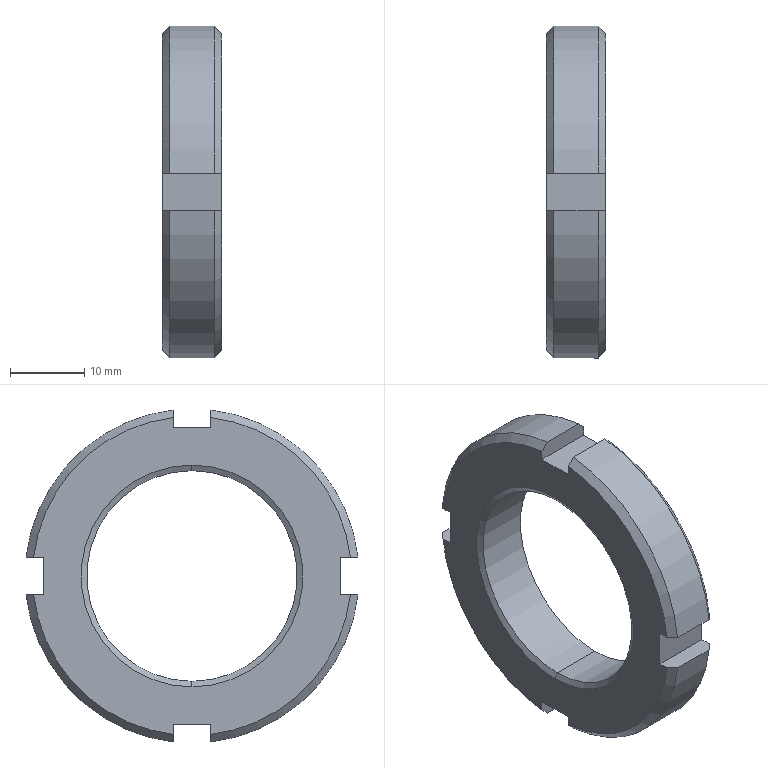Part | SolidWorks | features BaseBody 1 | 1 solid | 32 faces | box 8 x 44.721 x 44.721 mm | volume 7123 mm3 | plane 14 | cone 12 | cylinder 6 | commonest cylinder face diameters 45 x4 28.376 x2
STEP:
#1=CARTESIAN_POINT('',(0.433,0.,-14.188));
#2=VERTEX_POINT('',#1);
#3=CARTESIAN_POINT('',(0.433,0.,14.188));
#4=VERTEX_POINT('',#3);
#5=CARTESIAN_POINT('',(0.433,0.,0.));
#6=DIRECTION('',(-1.,0.,0.));
#7=DIRECTION('',(0.,0.,-1.));
#8=AXIS2_PLACEMENT_3D('',#5,#6,#7);
#9=CIRCLE('',#8,14.188);
#10=EDGE_CURVE('',#2,#4,#9,.T.);
#11=ORIENTED_EDGE('',*,*,#10,.F.);
#12=CARTESIAN_POINT('',(0.,0.,-14.938));
#13=VERTEX_POINT('',#12);
#14=CARTESIAN_POINT('',(0.,0.,-14.938));
#15=DIRECTION('',(-0.5,0.,-0.866));
#16=VECTOR('',#15,1000.);
#17=LINE('',#14,#16);
#18=EDGE_CURVE('',#2,#13,#17,.T.);
#19=ORIENTED_EDGE('',*,*,#18,.T.);
#20=CARTESIAN_POINT('',(0.,0.,14.938));
#21=VERTEX_POINT('',#20);
#22=CARTESIAN_POINT('',(0.,0.,0.));
#23=DIRECTION('',(1.,0.,0.));
#24=DIRECTION('',(0.,0.,1.));
#25=AXIS2_PLACEMENT_3D('',#22,#23,#24);
#26=CIRCLE('',#25,14.938);
#27=EDGE_CURVE('',#21,#13,#26,.T.);
#28=ORIENTED_EDGE('',*,*,#27,.F.);
#29=CARTESIAN_POINT('',(0.,0.,14.938));
#30=DIRECTION('',(-0.5,0.,0.866));
#31=VECTOR('',#30,1000.);
#32=LINE('',#29,#31);
#33=EDGE_CURVE('',#4,#21,#32,.T.);
#34=ORIENTED_EDGE('',*,*,#33,.F.);
#35=EDGE_LOOP('',(#11,#19,#28,#34));
#36=FACE_OUTER_BOUND('',#35,.T.);
#37=CARTESIAN_POINT('',(0.,0.,0.));
#38=DIRECTION('',(-1.,0.,0.));
#39=DIRECTION('',(0.,0.,1.));
#40=AXIS2_PLACEMENT_3D('',#37,#38,#39);
#41=CONICAL_SURFACE('',#40,14.938,1.047);
#42=ADVANCED_FACE('',(#36),#41,.F.);
#43=CARTESIAN_POINT('',(7.567,0.,-14.188));
#44=VERTEX_POINT('',#43);
#45=CARTESIAN_POINT('',(7.567,0.,14.188));
#46=VERTEX_POINT('',#45);
#47=CARTESIAN_POINT('',(7.567,0.,0.));
#48=DIRECTION('',(-1.,0.,0.));
#49=DIRECTION('',(0.,0.,1.));
#50=AXIS2_PLACEMENT_3D('',#47,#48,#49);
#51=CIRCLE('',#50,14.188);
#52=EDGE_CURVE('',#44,#46,#51,.T.);
#53=ORIENTED_EDGE('',*,*,#52,.F.);
#54=CARTESIAN_POINT('',(64.14,0.,-14.188));
#55=DIRECTION('',(-1.,0.,0.));
#56=VECTOR('',#55,1000.);
#57=LINE('',#54,#56);
#58=EDGE_CURVE('',#44,#2,#57,.T.);
#59=ORIENTED_EDGE('',*,*,#58,.T.);
#60=ORIENTED_EDGE('',*,*,#10,.T.);
#61=CARTESIAN_POINT('',(64.14,0.,14.188));
#62=DIRECTION('',(-1.,0.,0.));
#63=VECTOR('',#62,1000.);
#64=LINE('',#61,#63);
#65=EDGE_CURVE('',#46,#4,#64,.T.);
#66=ORIENTED_EDGE('',*,*,#65,.F.);
#67=EDGE_LOOP('',(#53,#59,#60,#66));
#68=FACE_OUTER_BOUND('',#67,.T.);
#69=CARTESIAN_POINT('',(64.14,0.,0.));
#70=DIRECTION('',(-1.,0.,0.));
#71=DIRECTION('',(0.,0.,1.));
#72=AXIS2_PLACEMENT_3D('',#69,#70,#71);
#73=CYLINDRICAL_SURFACE('',#72,14.188);
#74=ADVANCED_FACE('',(#68),#73,.F.);
#75=ORIENTED_EDGE('',*,*,#52,.T.);
#76=CARTESIAN_POINT('',(8.,0.,14.938));
#77=VERTEX_POINT('',#76);
#78=CARTESIAN_POINT('',(8.,0.,14.938));
#79=DIRECTION('',(0.5,0.,0.866));
#80=VECTOR('',#79,1000.);
#81=LINE('',#78,#80);
#82=EDGE_CURVE('',#46,#77,#81,.T.);
#83=ORIENTED_EDGE('',*,*,#82,.T.);
#84=CARTESIAN_POINT('',(8.,0.,-14.938));
#85=VERTEX_POINT('',#84);
#86=CARTESIAN_POINT('',(8.,0.,0.));
#87=DIRECTION('',(-1.,0.,0.));
#88=DIRECTION('',(0.,0.,-1.));
#89=AXIS2_PLACEMENT_3D('',#86,#87,#88);
#90=CIRCLE('',#89,14.938);
#91=EDGE_CURVE('',#85,#77,#90,.T.);
#92=ORIENTED_EDGE('',*,*,#91,.F.);
#93=CARTESIAN_POINT('',(8.,0.,-14.938));
#94=DIRECTION('',(0.5,0.,-0.866));
#95=VECTOR('',#94,1000.);
#96=LINE('',#93,#95);
#97=EDGE_CURVE('',#44,#85,#96,.T.);
#98=ORIENTED_EDGE('',*,*,#97,.F.);
#99=EDGE_LOOP('',(#75,#83,#92,#98));
#100=FACE_OUTER_BOUND('',#99,.T.);
#101=CARTESIAN_POINT('',(8.,0.,0.));
#102=DIRECTION('',(1.,0.,0.));
#103=DIRECTION('',(0.,0.,-1.));
#104=AXIS2_PLACEMENT_3D('',#101,#102,#103);
#105=CONICAL_SURFACE('',#104,14.938,1.047);
#106=ADVANCED_FACE('',(#100),#105,.F.);
#107=ORIENTED_EDGE('',*,*,#27,.T.);
#108=CARTESIAN_POINT('',(0.,0.,0.));
#109=DIRECTION('',(1.,0.,0.));
#110=DIRECTION('',(0.,0.,1.));
#111=AXIS2_PLACEMENT_3D('',#108,#109,#110);
#112=CIRCLE('',#111,14.938);
#113=EDGE_CURVE('',#13,#21,#112,.T.);
#114=ORIENTED_EDGE('',*,*,#113,.T.);
#115=EDGE_LOOP('',(#107,#114));
#116=FACE_BOUND('',#115,.T.);
#117=CARTESIAN_POINT('',(0.,-20.,-2.5));
#118=VERTEX_POINT('',#117);
#119=CARTESIAN_POINT('',(0.,-20.,2.5));
#120=VERTEX_POINT('',#119);
#121=CARTESIAN_POINT('',(0.,-20.,0.));
#122=DIRECTION('',(0.,0.,1.));
#123=VECTOR('',#122,1000.);
#124=LINE('',#121,#123);
#125=EDGE_CURVE('',#118,#120,#124,.T.);
#126=ORIENTED_EDGE('',*,*,#125,.T.);
#127=CARTESIAN_POINT('',(0.,-21.354,2.5));
#128=VERTEX_POINT('',#127);
#129=CARTESIAN_POINT('',(0.,-20.,2.5));
#130=DIRECTION('',(0.,-1.,0.));
#131=VECTOR('',#130,1000.);
#132=LINE('',#129,#131);
#133=EDGE_CURVE('',#120,#128,#132,.T.);
#134=ORIENTED_EDGE('',*,*,#133,.T.);
#135=CARTESIAN_POINT('',(0.,-2.5,21.354));
#136=VERTEX_POINT('',#135);
#137=CARTESIAN_POINT('',(0.,0.,0.));
#138=DIRECTION('',(-1.,0.,0.));
#139=DIRECTION('',(0.,0.,-1.));
#140=AXIS2_PLACEMENT_3D('',#137,#138,#139);
#141=CIRCLE('',#140,21.5);
#142=EDGE_CURVE('',#128,#136,#141,.T.);
#143=ORIENTED_EDGE('',*,*,#142,.T.);
#144=CARTESIAN_POINT('',(0.,-2.5,20.));
#145=VERTEX_POINT('',#144);
#146=CARTESIAN_POINT('',(0.,-2.5,22.361));
#147=DIRECTION('',(0.,0.,-1.));
#148=VECTOR('',#147,1000.);
#149=LINE('',#146,#148);
#150=EDGE_CURVE('',#136,#145,#149,.T.);
#151=ORIENTED_EDGE('',*,*,#150,.T.);
#152=CARTESIAN_POINT('',(0.,2.5,20.));
#153=VERTEX_POINT('',#152);
#154=CARTESIAN_POINT('',(0.,11.25,20.));
#155=DIRECTION('',(0.,1.,0.));
#156=VECTOR('',#155,1000.);
#157=LINE('',#154,#156);
#158=EDGE_CURVE('',#145,#153,#157,.T.);
#159=ORIENTED_EDGE('',*,*,#158,.T.);
#160=CARTESIAN_POINT('',(0.,2.5,21.354));
#161=VERTEX_POINT('',#160);
#162=CARTESIAN_POINT('',(0.,2.5,20.));
#163=DIRECTION('',(0.,0.,1.));
#164=VECTOR('',#163,1000.);
#165=LINE('',#162,#164);
#166=EDGE_CURVE('',#153,#161,#165,.T.);
#167=ORIENTED_EDGE('',*,*,#166,.T.);
#168=CARTESIAN_POINT('',(0.,21.354,2.5));
#169=VERTEX_POINT('',#168);
#170=CARTESIAN_POINT('',(0.,0.,0.));
#171=DIRECTION('',(-1.,0.,0.));
#172=DIRECTION('',(0.,0.,-1.));
#173=AXIS2_PLACEMENT_3D('',#170,#171,#172);
#174=CIRCLE('',#173,21.5);
#175=EDGE_CURVE('',#161,#169,#174,.T.);
#176=ORIENTED_EDGE('',*,*,#175,.T.);
#177=CARTESIAN_POINT('',(0.,20.,2.5));
#178=VERTEX_POINT('',#177);
#179=CARTESIAN_POINT('',(0.,22.361,2.5));
#180=DIRECTION('',(0.,-1.,0.));
#181=VECTOR('',#180,1000.);
#182=LINE('',#179,#181);
#183=EDGE_CURVE('',#169,#178,#182,.T.);
#184=ORIENTED_EDGE('',*,*,#183,.T.);
#185=CARTESIAN_POINT('',(0.,20.,-2.5));
#186=VERTEX_POINT('',#185);
#187=CARTESIAN_POINT('',(0.,20.,0.));
#188=DIRECTION('',(0.,0.,-1.));
#189=VECTOR('',#188,1000.);
#190=LINE('',#187,#189);
#191=EDGE_CURVE('',#178,#186,#190,.T.);
#192=ORIENTED_EDGE('',*,*,#191,.T.);
#193=CARTESIAN_POINT('',(0.,21.354,-2.5));
#194=VERTEX_POINT('',#193);
#195=CARTESIAN_POINT('',(0.,20.,-2.5));
#196=DIRECTION('',(0.,1.,0.));
#197=VECTOR('',#196,1000.);
#198=LINE('',#195,#197);
#199=EDGE_CURVE('',#186,#194,#198,.T.);
#200=ORIENTED_EDGE('',*,*,#199,.T.);
#201=CARTESIAN_POINT('',(0.,2.5,-21.354));
#202=VERTEX_POINT('',#201);
#203=CARTESIAN_POINT('',(0.,0.,0.));
#204=DIRECTION('',(-1.,0.,0.));
#205=DIRECTION('',(0.,0.,-1.));
#206=AXIS2_PLACEMENT_3D('',#203,#204,#205);
#207=CIRCLE('',#206,21.5);
#208=EDGE_CURVE('',#194,#202,#207,.T.);
#209=ORIENTED_EDGE('',*,*,#208,.T.);
#210=CARTESIAN_POINT('',(0.,2.5,-20.));
#211=VERTEX_POINT('',#210);
#212=CARTESIAN_POINT('',(0.,2.5,-22.361));
#213=DIRECTION('',(0.,0.,1.));
#214=VECTOR('',#213,1000.);
#215=LINE('',#212,#214);
#216=EDGE_CURVE('',#202,#211,#215,.T.);
#217=ORIENTED_EDGE('',*,*,#216,.T.);
#218=CARTESIAN_POINT('',(0.,-2.5,-20.));
#219=VERTEX_POINT('',#218);
#220=CARTESIAN_POINT('',(0.,11.25,-20.));
#221=DIRECTION('',(0.,-1.,0.));
#222=VECTOR('',#221,1000.);
#223=LINE('',#220,#222);
#224=EDGE_CURVE('',#211,#219,#223,.T.);
#225=ORIENTED_EDGE('',*,*,#224,.T.);
#226=CARTESIAN_POINT('',(0.,-2.5,-21.354));
#227=VERTEX_POINT('',#226);
#228=CARTESIAN_POINT('',(0.,-2.5,-20.));
#229=DIRECTION('',(0.,0.,-1.));
#230=VECTOR('',#229,1000.);
#231=LINE('',#228,#230);
#232=EDGE_CURVE('',#219,#227,#231,.T.);
#233=ORIENTED_EDGE('',*,*,#232,.T.);
#234=CARTESIAN_POINT('',(0.,-21.354,-2.5));
#235=VERTEX_POINT('',#234);
#236=CARTESIAN_POINT('',(0.,0.,0.));
#237=DIRECTION('',(-1.,0.,0.));
#238=DIRECTION('',(0.,0.,-1.));
#239=AXIS2_PLACEMENT_3D('',#236,#237,#238);
#240=CIRCLE('',#239,21.5);
#241=EDGE_CURVE('',#227,#235,#240,.T.);
#242=ORIENTED_EDGE('',*,*,#241,.T.);
#243=CARTESIAN_POINT('',(0.,-22.361,-2.5));
#244=DIRECTION('',(0.,1.,0.));
#245=VECTOR('',#244,1000.);
#246=LINE('',#243,#245);
#247=EDGE_CURVE('',#235,#118,#246,.T.);
#248=ORIENTED_EDGE('',*,*,#247,.T.);
#249=EDGE_LOOP('',(#126,#134,#143,#151,#159,#167,#176,#184,#192,#200,#209,#217,#225,#233,#242,#248));
#250=FACE_OUTER_BOUND('',#249,.T.);
#251=CARTESIAN_POINT('',(0.,11.25,0.));
#252=DIRECTION('',(-1.,0.,0.));
#253=DIRECTION('',(0.,0.,1.));
#254=AXIS2_PLACEMENT_3D('',#251,#252,#253);
#255=PLANE('',#254);
#256=ADVANCED_FACE('',(#116,#250),#255,.T.);
#257=ORIENTED_EDGE('',*,*,#18,.F.);
#258=CARTESIAN_POINT('',(0.433,0.,0.));
#259=DIRECTION('',(-1.,0.,0.));
#260=DIRECTION('',(0.,0.,-1.));
#261=AXIS2_PLACEMENT_3D('',#258,#259,#260);
#262=CIRCLE('',#261,14.188);
#263=EDGE_CURVE('',#4,#2,#262,.T.);
#264=ORIENTED_EDGE('',*,*,#263,.F.);
#265=ORIENTED_EDGE('',*,*,#33,.T.);
#266=ORIENTED_EDGE('',*,*,#113,.F.);
#267=EDGE_LOOP('',(#257,#264,#265,#266));
#268=FACE_OUTER_BOUND('',#267,.T.);
#269=CARTESIAN_POINT('',(0.,0.,0.));
#270=DIRECTION('',(-1.,0.,0.));
#271=DIRECTION('',(0.,0.,1.));
#272=AXIS2_PLACEMENT_3D('',#269,#270,#271);
#273=CONICAL_SURFACE('',#272,14.938,1.047);
#274=ADVANCED_FACE('',(#268),#273,.F.);
#275=CARTESIAN_POINT('',(8.,-20.,-2.5));
#276=VERTEX_POINT('',#275);
#277=CARTESIAN_POINT('',(8.,-20.,-2.5));
#278=DIRECTION('',(-1.,0.,0.));
#279=VECTOR('',#278,1000.);
#280=LINE('',#277,#279);
#281=EDGE_CURVE('',#276,#118,#280,.T.);
#282=ORIENTED_EDGE('',*,*,#281,.F.);
#283=CARTESIAN_POINT('',(8.,-20.,2.5));
#284=VERTEX_POINT('',#283);
#285=CARTESIAN_POINT('',(8.,-20.,-2.5));
#286=DIRECTION('',(0.,0.,-1.));
#287=VECTOR('',#286,1000.);
#288=LINE('',#285,#287);
#289=EDGE_CURVE('',#284,#276,#288,.T.);
#290=ORIENTED_EDGE('',*,*,#289,.F.);
#291=CARTESIAN_POINT('',(8.,-20.,2.5));
#292=DIRECTION('',(1.,0.,0.));
#293=VECTOR('',#292,1000.);
#294=LINE('',#291,#293);
#295=EDGE_CURVE('',#120,#284,#294,.T.);
#296=ORIENTED_EDGE('',*,*,#295,.F.);
#297=ORIENTED_EDGE('',*,*,#125,.F.);
#298=EDGE_LOOP('',(#282,#290,#296,#297));
#299=FACE_OUTER_BOUND('',#298,.T.);
#300=CARTESIAN_POINT('',(8.,-20.,-2.5));
#301=DIRECTION('',(0.,1.,0.));
#302=DIRECTION('',(0.,0.,1.));
#303=AXIS2_PLACEMENT_3D('',#300,#301,#302);
#304=PLANE('',#303);
#305=ADVANCED_FACE('',(#299),#304,.F.);
#306=CARTESIAN_POINT('',(1.,-22.361,-2.5));
#307=VERTEX_POINT('',#306);
#308=CARTESIAN_POINT('',(1.,-22.361,-2.5));
#309=CARTESIAN_POINT('',(0.6666,-22.025,-2.5));
#310=CARTESIAN_POINT('',(0.3333,-21.69,-2.5));
#311=CARTESIAN_POINT('',(0.,-21.354,-2.5));
#312=B_SPLINE_CURVE_WITH_KNOTS('',3,(#308,#309,#310,#311),.UNSPECIFIED.,.F.,.F.,(4,4),(0.,0.001419),.UNSPECIFIED.);
#313=EDGE_CURVE('',#307,#235,#312,.T.);
#314=ORIENTED_EDGE('',*,*,#313,.T.);
#315=ORIENTED_EDGE('',*,*,#241,.F.);
#316=CARTESIAN_POINT('',(1.,-2.5,-22.361));
#317=VERTEX_POINT('',#316);
#318=CARTESIAN_POINT('',(0.,-2.5,-21.354));
#319=CARTESIAN_POINT('',(0.3333,-2.5,-21.69));
#320=CARTESIAN_POINT('',(0.6666,-2.5,-22.025));
#321=CARTESIAN_POINT('',(1.,-2.5,-22.361));
#322=B_SPLINE_CURVE_WITH_KNOTS('',3,(#318,#319,#320,#321),.UNSPECIFIED.,.F.,.F.,(4,4),(0.,0.001419),.UNSPECIFIED.);
#323=EDGE_CURVE('',#227,#317,#322,.T.);
#324=ORIENTED_EDGE('',*,*,#323,.T.);
#325=CARTESIAN_POINT('',(1.,0.,0.));
#326=DIRECTION('',(-1.,0.,0.));
#327=DIRECTION('',(0.,-1.,0.));
#328=AXIS2_PLACEMENT_3D('',#325,#326,#327);
#329=CIRCLE('',#328,22.5);
#330=EDGE_CURVE('',#317,#307,#329,.T.);
#331=ORIENTED_EDGE('',*,*,#330,.T.);
#332=EDGE_LOOP('',(#314,#315,#324,#331));
#333=FACE_OUTER_BOUND('',#332,.T.);
#334=CARTESIAN_POINT('',(1.,0.,0.));
#335=DIRECTION('',(1.,0.,0.));
#336=DIRECTION('',(0.,0.,-1.));
#337=AXIS2_PLACEMENT_3D('',#334,#335,#336);
#338=CONICAL_SURFACE('',#337,22.5,0.7854);
#339=ADVANCED_FACE('',(#333),#338,.T.);
#340=CARTESIAN_POINT('',(8.,2.5,-20.));
#341=VERTEX_POINT('',#340);
#342=CARTESIAN_POINT('',(8.,2.5,-20.));
#343=DIRECTION('',(-1.,0.,0.));
#344=VECTOR('',#343,1000.);
#345=LINE('',#342,#344);
#346=EDGE_CURVE('',#341,#211,#345,.T.);
#347=ORIENTED_EDGE('',*,*,#346,.F.);
#348=CARTESIAN_POINT('',(8.,-2.5,-20.));
#349=VERTEX_POINT('',#348);
#350=CARTESIAN_POINT('',(8.,2.5,-20.));
#351=DIRECTION('',(0.,1.,0.));
#352=VECTOR('',#351,1000.);
#353=LINE('',#350,#352);
#354=EDGE_CURVE('',#349,#341,#353,.T.);
#355=ORIENTED_EDGE('',*,*,#354,.F.);
#356=CARTESIAN_POINT('',(8.,-2.5,-20.));
#357=DIRECTION('',(1.,0.,0.));
#358=VECTOR('',#357,1000.);
#359=LINE('',#356,#358);
#360=EDGE_CURVE('',#219,#349,#359,.T.);
#361=ORIENTED_EDGE('',*,*,#360,.F.);
#362=ORIENTED_EDGE('',*,*,#224,.F.);
#363=EDGE_LOOP('',(#347,#355,#361,#362));
#364=FACE_OUTER_BOUND('',#363,.T.);
#365=CARTESIAN_POINT('',(8.,2.5,-20.));
#366=DIRECTION('',(0.,0.,1.));
#367=DIRECTION('',(0.,-1.,0.));
#368=AXIS2_PLACEMENT_3D('',#365,#366,#367);
#369=PLANE('',#368);
#370=ADVANCED_FACE('',(#364),#369,.F.);
#371=CARTESIAN_POINT('',(1.,2.5,-22.361));
#372=VERTEX_POINT('',#371);
#373=CARTESIAN_POINT('',(1.,2.5,-22.361));
#374=CARTESIAN_POINT('',(0.6666,2.5,-22.025));
#375=CARTESIAN_POINT('',(0.3333,2.5,-21.69));
#376=CARTESIAN_POINT('',(0.,2.5,-21.354));
#377=B_SPLINE_CURVE_WITH_KNOTS('',3,(#373,#374,#375,#376),.UNSPECIFIED.,.F.,.F.,(4,4),(0.,0.001419),.UNSPECIFIED.);
#378=EDGE_CURVE('',#372,#202,#377,.T.);
#379=ORIENTED_EDGE('',*,*,#378,.T.);
#380=ORIENTED_EDGE('',*,*,#208,.F.);
#381=CARTESIAN_POINT('',(1.,22.361,-2.5));
#382=VERTEX_POINT('',#381);
#383=CARTESIAN_POINT('',(0.,21.354,-2.5));
#384=CARTESIAN_POINT('',(0.3333,21.69,-2.5));
#385=CARTESIAN_POINT('',(0.6666,22.025,-2.5));
#386=CARTESIAN_POINT('',(1.,22.361,-2.5));
#387=B_SPLINE_CURVE_WITH_KNOTS('',3,(#383,#384,#385,#386),.UNSPECIFIED.,.F.,.F.,(4,4),(0.,0.001419),.UNSPECIFIED.);
#388=EDGE_CURVE('',#194,#382,#387,.T.);
#389=ORIENTED_EDGE('',*,*,#388,.T.);
#390=CARTESIAN_POINT('',(1.,0.,0.));
#391=DIRECTION('',(-1.,0.,0.));
#392=DIRECTION('',(0.,1.,0.));
#393=AXIS2_PLACEMENT_3D('',#390,#391,#392);
#394=CIRCLE('',#393,22.5);
#395=EDGE_CURVE('',#382,#372,#394,.T.);
#396=ORIENTED_EDGE('',*,*,#395,.T.);
#397=EDGE_LOOP('',(#379,#380,#389,#396));
#398=FACE_OUTER_BOUND('',#397,.T.);
#399=CARTESIAN_POINT('',(1.,0.,0.));
#400=DIRECTION('',(1.,0.,0.));
#401=DIRECTION('',(0.,0.,-1.));
#402=AXIS2_PLACEMENT_3D('',#399,#400,#401);
#403=CONICAL_SURFACE('',#402,22.5,0.7854);
#404=ADVANCED_FACE('',(#398),#403,.T.);
#405=CARTESIAN_POINT('',(8.,20.,2.5));
#406=VERTEX_POINT('',#405);
#407=CARTESIAN_POINT('',(8.,20.,2.5));
#408=DIRECTION('',(-1.,0.,0.));
#409=VECTOR('',#408,1000.);
#410=LINE('',#407,#409);
#411=EDGE_CURVE('',#406,#178,#410,.T.);
#412=ORIENTED_EDGE('',*,*,#411,.F.);
#413=CARTESIAN_POINT('',(8.,20.,-2.5));
#414=VERTEX_POINT('',#413);
#415=CARTESIAN_POINT('',(8.,20.,2.5));
#416=DIRECTION('',(0.,0.,1.));
#417=VECTOR('',#416,1000.);
#418=LINE('',#415,#417);
#419=EDGE_CURVE('',#414,#406,#418,.T.);
#420=ORIENTED_EDGE('',*,*,#419,.F.);
#421=CARTESIAN_POINT('',(8.,20.,-2.5));
#422=DIRECTION('',(1.,0.,0.));
#423=VECTOR('',#422,1000.);
#424=LINE('',#421,#423);
#425=EDGE_CURVE('',#186,#414,#424,.T.);
#426=ORIENTED_EDGE('',*,*,#425,.F.);
#427=ORIENTED_EDGE('',*,*,#191,.F.);
#428=EDGE_LOOP('',(#412,#420,#426,#427));
#429=FACE_OUTER_BOUND('',#428,.T.);
#430=CARTESIAN_POINT('',(8.,20.,2.5));
#431=DIRECTION('',(0.,-1.,0.));
#432=DIRECTION('',(0.,0.,-1.));
#433=AXIS2_PLACEMENT_3D('',#430,#431,#432);
#434=PLANE('',#433);
#435=ADVANCED_FACE('',(#429),#434,.F.);
#436=CARTESIAN_POINT('',(1.,22.361,2.5));
#437=VERTEX_POINT('',#436);
#438=CARTESIAN_POINT('',(1.,22.361,2.5));
#439=CARTESIAN_POINT('',(0.6666,22.025,2.5));
#440=CARTESIAN_POINT('',(0.3333,21.69,2.5));
#441=CARTESIAN_POINT('',(0.,21.354,2.5));
#442=B_SPLINE_CURVE_WITH_KNOTS('',3,(#438,#439,#440,#441),.UNSPECIFIED.,.F.,.F.,(4,4),(0.,0.001419),.UNSPECIFIED.);
#443=EDGE_CURVE('',#437,#169,#442,.T.);
#444=ORIENTED_EDGE('',*,*,#443,.T.);
#445=ORIENTED_EDGE('',*,*,#175,.F.);
#446=CARTESIAN_POINT('',(1.,2.5,22.361));
#447=VERTEX_POINT('',#446);
#448=CARTESIAN_POINT('',(0.,2.5,21.354));
#449=CARTESIAN_POINT('',(0.3333,2.5,21.69));
#450=CARTESIAN_POINT('',(0.6666,2.5,22.025));
#451=CARTESIAN_POINT('',(1.,2.5,22.361));
#452=B_SPLINE_CURVE_WITH_KNOTS('',3,(#448,#449,#450,#451),.UNSPECIFIED.,.F.,.F.,(4,4),(0.,0.001419),.UNSPECIFIED.);
#453=EDGE_CURVE('',#161,#447,#452,.T.);
#454=ORIENTED_EDGE('',*,*,#453,.T.);
#455=CARTESIAN_POINT('',(1.,0.,0.));
#456=DIRECTION('',(-1.,0.,0.));
#457=DIRECTION('',(0.,1.,0.));
#458=AXIS2_PLACEMENT_3D('',#455,#456,#457);
#459=CIRCLE('',#458,22.5);
#460=EDGE_CURVE('',#447,#437,#459,.T.);
#461=ORIENTED_EDGE('',*,*,#460,.T.);
#462=EDGE_LOOP('',(#444,#445,#454,#461));
#463=FACE_OUTER_BOUND('',#462,.T.);
#464=CARTESIAN_POINT('',(1.,0.,0.));
#465=DIRECTION('',(1.,0.,0.));
#466=DIRECTION('',(0.,0.,-1.));
#467=AXIS2_PLACEMENT_3D('',#464,#465,#466);
#468=CONICAL_SURFACE('',#467,22.5,0.7854);
#469=ADVANCED_FACE('',(#463),#468,.T.);
#470=CARTESIAN_POINT('',(8.,-2.5,20.));
#471=VERTEX_POINT('',#470);
#472=CARTESIAN_POINT('',(8.,-2.5,20.));
#473=DIRECTION('',(-1.,0.,0.));
#474=VECTOR('',#473,1000.);
#475=LINE('',#472,#474);
#476=EDGE_CURVE('',#471,#145,#475,.T.);
#477=ORIENTED_EDGE('',*,*,#476,.F.);
#478=CARTESIAN_POINT('',(8.,2.5,20.));
#479=VERTEX_POINT('',#478);
#480=CARTESIAN_POINT('',(8.,-2.5,20.));
#481=DIRECTION('',(0.,-1.,0.));
#482=VECTOR('',#481,1000.);
#483=LINE('',#480,#482);
#484=EDGE_CURVE('',#479,#471,#483,.T.);
#485=ORIENTED_EDGE('',*,*,#484,.F.);
#486=CARTESIAN_POINT('',(8.,2.5,20.));
#487=DIRECTION('',(1.,0.,0.));
#488=VECTOR('',#487,1000.);
#489=LINE('',#486,#488);
#490=EDGE_CURVE('',#153,#479,#489,.T.);
#491=ORIENTED_EDGE('',*,*,#490,.F.);
#492=ORIENTED_EDGE('',*,*,#158,.F.);
#493=EDGE_LOOP('',(#477,#485,#491,#492));
#494=FACE_OUTER_BOUND('',#493,.T.);
#495=CARTESIAN_POINT('',(8.,-2.5,20.));
#496=DIRECTION('',(0.,0.,-1.));
#497=DIRECTION('',(0.,1.,0.));
#498=AXIS2_PLACEMENT_3D('',#495,#496,#497);
#499=PLANE('',#498);
#500=ADVANCED_FACE('',(#494),#499,.F.);
#501=CARTESIAN_POINT('',(1.,-2.5,22.361));
#502=VERTEX_POINT('',#501);
#503=CARTESIAN_POINT('',(1.,-2.5,22.361));
#504=CARTESIAN_POINT('',(0.6666,-2.5,22.025));
#505=CARTESIAN_POINT('',(0.3333,-2.5,21.69));
#506=CARTESIAN_POINT('',(0.,-2.5,21.354));
#507=B_SPLINE_CURVE_WITH_KNOTS('',3,(#503,#504,#505,#506),.UNSPECIFIED.,.F.,.F.,(4,4),(0.,0.001419),.UNSPECIFIED.);
#508=EDGE_CURVE('',#502,#136,#507,.T.);
#509=ORIENTED_EDGE('',*,*,#508,.T.);
#510=ORIENTED_EDGE('',*,*,#142,.F.);
#511=CARTESIAN_POINT('',(1.,-22.361,2.5));
#512=VERTEX_POINT('',#511);
#513=CARTESIAN_POINT('',(0.,-21.354,2.5));
#514=CARTESIAN_POINT('',(0.3333,-21.69,2.5));
#515=CARTESIAN_POINT('',(0.6666,-22.025,2.5));
#516=CARTESIAN_POINT('',(1.,-22.361,2.5));
#517=B_SPLINE_CURVE_WITH_KNOTS('',3,(#513,#514,#515,#516),.UNSPECIFIED.,.F.,.F.,(4,4),(0.,0.001419),.UNSPECIFIED.);
#518=EDGE_CURVE('',#128,#512,#517,.T.);
#519=ORIENTED_EDGE('',*,*,#518,.T.);
#520=CARTESIAN_POINT('',(1.,0.,0.));
#521=DIRECTION('',(-1.,0.,0.));
#522=DIRECTION('',(0.,-1.,0.));
#523=AXIS2_PLACEMENT_3D('',#520,#521,#522);
#524=CIRCLE('',#523,22.5);
#525=EDGE_CURVE('',#512,#502,#524,.T.);
#526=ORIENTED_EDGE('',*,*,#525,.T.);
#527=EDGE_LOOP('',(#509,#510,#519,#526));
#528=FACE_OUTER_BOUND('',#527,.T.);
#529=CARTESIAN_POINT('',(1.,0.,0.));
#530=DIRECTION('',(1.,0.,0.));
#531=DIRECTION('',(0.,0.,-1.));
#532=AXIS2_PLACEMENT_3D('',#529,#530,#531);
#533=CONICAL_SURFACE('',#532,22.5,0.7854);
#534=ADVANCED_FACE('',(#528),#533,.T.);
#535=ORIENTED_EDGE('',*,*,#58,.F.);
#536=CARTESIAN_POINT('',(7.567,0.,0.));
#537=DIRECTION('',(-1.,0.,0.));
#538=DIRECTION('',(0.,0.,1.));
#539=AXIS2_PLACEMENT_3D('',#536,#537,#538);
#540=CIRCLE('',#539,14.188);
#541=EDGE_CURVE('',#46,#44,#540,.T.);
#542=ORIENTED_EDGE('',*,*,#541,.F.);
#543=ORIENTED_EDGE('',*,*,#65,.T.);
#544=ORIENTED_EDGE('',*,*,#263,.T.);
#545=EDGE_LOOP('',(#535,#542,#543,#544));
#546=FACE_OUTER_BOUND('',#545,.T.);
#547=CARTESIAN_POINT('',(64.14,0.,0.));
#548=DIRECTION('',(-1.,0.,0.));
#549=DIRECTION('',(0.,0.,1.));
#550=AXIS2_PLACEMENT_3D('',#547,#548,#549);
#551=CYLINDRICAL_SURFACE('',#550,14.188);
#552=ADVANCED_FACE('',(#546),#551,.F.);
#553=CARTESIAN_POINT('',(8.,-21.354,-2.5));
#554=VERTEX_POINT('',#553);
#555=CARTESIAN_POINT('',(8.,-22.361,-2.5));
#556=DIRECTION('',(0.,-1.,0.));
#557=VECTOR('',#556,1000.);
#558=LINE('',#555,#557);
#559=EDGE_CURVE('',#276,#554,#558,.T.);
#560=ORIENTED_EDGE('',*,*,#559,.F.);
#561=ORIENTED_EDGE('',*,*,#281,.T.);
#562=ORIENTED_EDGE('',*,*,#247,.F.);
#563=ORIENTED_EDGE('',*,*,#313,.F.);
#564=CARTESIAN_POINT('',(7.,-22.361,-2.5));
#565=VERTEX_POINT('',#564);
#566=CARTESIAN_POINT('',(8.,-22.361,-2.5));
#567=DIRECTION('',(-1.,0.,0.));
#568=VECTOR('',#567,1000.);
#569=LINE('',#566,#568);
#570=EDGE_CURVE('',#565,#307,#569,.T.);
#571=ORIENTED_EDGE('',*,*,#570,.F.);
#572=CARTESIAN_POINT('',(8.,-21.354,-2.5));
#573=CARTESIAN_POINT('',(7.667,-21.69,-2.5));
#574=CARTESIAN_POINT('',(7.333,-22.025,-2.5));
#575=CARTESIAN_POINT('',(7.,-22.361,-2.5));
#576=B_SPLINE_CURVE_WITH_KNOTS('',3,(#572,#573,#574,#575),.UNSPECIFIED.,.F.,.F.,(4,4),(0.,0.001419),.UNSPECIFIED.);
#577=EDGE_CURVE('',#554,#565,#576,.T.);
#578=ORIENTED_EDGE('',*,*,#577,.F.);
#579=EDGE_LOOP('',(#560,#561,#562,#563,#571,#578));
#580=FACE_OUTER_BOUND('',#579,.T.);
#581=CARTESIAN_POINT('',(8.,-22.361,-2.5));
#582=DIRECTION('',(0.,0.,-1.));
#583=DIRECTION('',(0.,1.,0.));
#584=AXIS2_PLACEMENT_3D('',#581,#582,#583);
#585=PLANE('',#584);
#586=ADVANCED_FACE('',(#580),#585,.F.);
#587=ORIENTED_EDGE('',*,*,#91,.T.);
#588=CARTESIAN_POINT('',(8.,0.,0.));
#589=DIRECTION('',(-1.,0.,0.));
#590=DIRECTION('',(0.,0.,-1.));
#591=AXIS2_PLACEMENT_3D('',#588,#589,#590);
#592=CIRCLE('',#591,14.938);
#593=EDGE_CURVE('',#77,#85,#592,.T.);
#594=ORIENTED_EDGE('',*,*,#593,.T.);
#595=EDGE_LOOP('',(#587,#594));
#596=FACE_BOUND('',#595,.T.);
#597=ORIENTED_EDGE('',*,*,#354,.T.);
#598=CARTESIAN_POINT('',(8.,2.5,-21.354));
#599=VERTEX_POINT('',#598);
#600=CARTESIAN_POINT('',(8.,2.5,0.));
#601=DIRECTION('',(0.,0.,-1.));
#602=VECTOR('',#601,1000.);
#603=LINE('',#600,#602);
#604=EDGE_CURVE('',#341,#599,#603,.T.);
#605=ORIENTED_EDGE('',*,*,#604,.T.);
#606=CARTESIAN_POINT('',(8.,21.354,-2.5));
#607=VERTEX_POINT('',#606);
#608=CARTESIAN_POINT('',(8.,0.,0.));
#609=DIRECTION('',(1.,0.,0.));
#610=DIRECTION('',(0.,0.,1.));
#611=AXIS2_PLACEMENT_3D('',#608,#609,#610);
#612=CIRCLE('',#611,21.5);
#613=EDGE_CURVE('',#599,#607,#612,.T.);
#614=ORIENTED_EDGE('',*,*,#613,.T.);
#615=CARTESIAN_POINT('',(8.,11.25,-2.5));
#616=DIRECTION('',(0.,-1.,0.));
#617=VECTOR('',#616,1000.);
#618=LINE('',#615,#617);
#619=EDGE_CURVE('',#607,#414,#618,.T.);
#620=ORIENTED_EDGE('',*,*,#619,.T.);
#621=ORIENTED_EDGE('',*,*,#419,.T.);
#622=CARTESIAN_POINT('',(8.,21.354,2.5));
#623=VERTEX_POINT('',#622);
#624=CARTESIAN_POINT('',(8.,11.25,2.5));
#625=DIRECTION('',(0.,1.,0.));
#626=VECTOR('',#625,1000.);
#627=LINE('',#624,#626);
#628=EDGE_CURVE('',#406,#623,#627,.T.);
#629=ORIENTED_EDGE('',*,*,#628,.T.);
#630=CARTESIAN_POINT('',(8.,2.5,21.354));
#631=VERTEX_POINT('',#630);
#632=CARTESIAN_POINT('',(8.,0.,0.));
#633=DIRECTION('',(1.,0.,0.));
#634=DIRECTION('',(0.,0.,1.));
#635=AXIS2_PLACEMENT_3D('',#632,#633,#634);
#636=CIRCLE('',#635,21.5);
#637=EDGE_CURVE('',#623,#631,#636,.T.);
#638=ORIENTED_EDGE('',*,*,#637,.T.);
#639=CARTESIAN_POINT('',(8.,2.5,0.));
#640=DIRECTION('',(0.,0.,-1.));
#641=VECTOR('',#640,1000.);
#642=LINE('',#639,#641);
#643=EDGE_CURVE('',#631,#479,#642,.T.);
#644=ORIENTED_EDGE('',*,*,#643,.T.);
#645=ORIENTED_EDGE('',*,*,#484,.T.);
#646=CARTESIAN_POINT('',(8.,-2.5,21.354));
#647=VERTEX_POINT('',#646);
#648=CARTESIAN_POINT('',(8.,-2.5,0.));
#649=DIRECTION('',(0.,0.,1.));
#650=VECTOR('',#649,1000.);
#651=LINE('',#648,#650);
#652=EDGE_CURVE('',#471,#647,#651,.T.);
#653=ORIENTED_EDGE('',*,*,#652,.T.);
#654=CARTESIAN_POINT('',(8.,-21.354,2.5));
#655=VERTEX_POINT('',#654);
#656=CARTESIAN_POINT('',(8.,0.,0.));
#657=DIRECTION('',(1.,0.,0.));
#658=DIRECTION('',(0.,0.,1.));
#659=AXIS2_PLACEMENT_3D('',#656,#657,#658);
#660=CIRCLE('',#659,21.5);
#661=EDGE_CURVE('',#647,#655,#660,.T.);
#662=ORIENTED_EDGE('',*,*,#661,.T.);
#663=CARTESIAN_POINT('',(8.,11.25,2.5));
#664=DIRECTION('',(0.,1.,0.));
#665=VECTOR('',#664,1000.);
#666=LINE('',#663,#665);
#667=EDGE_CURVE('',#655,#284,#666,.T.);
#668=ORIENTED_EDGE('',*,*,#667,.T.);
#669=ORIENTED_EDGE('',*,*,#289,.T.);
#670=ORIENTED_EDGE('',*,*,#559,.T.);
#671=CARTESIAN_POINT('',(8.,-2.5,-21.354));
#672=VERTEX_POINT('',#671);
#673=CARTESIAN_POINT('',(8.,0.,0.));
#674=DIRECTION('',(1.,0.,0.));
#675=DIRECTION('',(0.,0.,1.));
#676=AXIS2_PLACEMENT_3D('',#673,#674,#675);
#677=CIRCLE('',#676,21.5);
#678=EDGE_CURVE('',#554,#672,#677,.T.);
#679=ORIENTED_EDGE('',*,*,#678,.T.);
#680=CARTESIAN_POINT('',(8.,-2.5,0.));
#681=DIRECTION('',(0.,0.,1.));
#682=VECTOR('',#681,1000.);
#683=LINE('',#680,#682);
#684=EDGE_CURVE('',#672,#349,#683,.T.);
#685=ORIENTED_EDGE('',*,*,#684,.T.);
#686=EDGE_LOOP('',(#597,#605,#614,#620,#621,#629,#638,#644,#645,#653,#662,#668,#669,#670,#679,#685));
#687=FACE_OUTER_BOUND('',#686,.T.);
#688=CARTESIAN_POINT('',(8.,11.25,0.));
#689=DIRECTION('',(1.,0.,0.));
#690=DIRECTION('',(0.,0.,-1.));
#691=AXIS2_PLACEMENT_3D('',#688,#689,#690);
#692=PLANE('',#691);
#693=ADVANCED_FACE('',(#596,#687),#692,.T.);
#694=CARTESIAN_POINT('',(7.,-22.361,2.5));
#695=VERTEX_POINT('',#694);
#696=CARTESIAN_POINT('',(8.,-22.361,2.5));
#697=DIRECTION('',(1.,0.,0.));
#698=VECTOR('',#697,1000.);
#699=LINE('',#696,#698);
#700=EDGE_CURVE('',#512,#695,#699,.T.);
#701=ORIENTED_EDGE('',*,*,#700,.F.);
#702=ORIENTED_EDGE('',*,*,#518,.F.);
#703=ORIENTED_EDGE('',*,*,#133,.F.);
#704=ORIENTED_EDGE('',*,*,#295,.T.);
#705=ORIENTED_EDGE('',*,*,#667,.F.);
#706=CARTESIAN_POINT('',(7.,-22.361,2.5));
#707=CARTESIAN_POINT('',(7.333,-22.025,2.5));
#708=CARTESIAN_POINT('',(7.667,-21.69,2.5));
#709=CARTESIAN_POINT('',(8.,-21.354,2.5));
#710=B_SPLINE_CURVE_WITH_KNOTS('',3,(#706,#707,#708,#709),.UNSPECIFIED.,.F.,.F.,(4,4),(0.,0.001419),.UNSPECIFIED.);
#711=EDGE_CURVE('',#695,#655,#710,.T.);
#712=ORIENTED_EDGE('',*,*,#711,.F.);
#713=EDGE_LOOP('',(#701,#702,#703,#704,#705,#712));
#714=FACE_OUTER_BOUND('',#713,.T.);
#715=CARTESIAN_POINT('',(8.,-20.,2.5));
#716=DIRECTION('',(0.,0.,1.));
#717=DIRECTION('',(0.,-1.,0.));
#718=AXIS2_PLACEMENT_3D('',#715,#716,#717);
#719=PLANE('',#718);
#720=ADVANCED_FACE('',(#714),#719,.F.);
#721=ORIENTED_EDGE('',*,*,#330,.F.);
#722=CARTESIAN_POINT('',(7.,-2.5,-22.361));
#723=VERTEX_POINT('',#722);
#724=CARTESIAN_POINT('',(4.,-2.5,-22.361));
#725=DIRECTION('',(1.,0.,0.));
#726=VECTOR('',#725,1000.);
#727=LINE('',#724,#726);
#728=EDGE_CURVE('',#317,#723,#727,.T.);
#729=ORIENTED_EDGE('',*,*,#728,.T.);
#730=CARTESIAN_POINT('',(7.,0.,0.));
#731=DIRECTION('',(-1.,0.,0.));
#732=DIRECTION('',(0.,0.,-1.));
#733=AXIS2_PLACEMENT_3D('',#730,#731,#732);
#734=CIRCLE('',#733,22.5);
#735=EDGE_CURVE('',#723,#565,#734,.T.);
#736=ORIENTED_EDGE('',*,*,#735,.T.);
#737=ORIENTED_EDGE('',*,*,#570,.T.);
#738=EDGE_LOOP('',(#721,#729,#736,#737));
#739=FACE_OUTER_BOUND('',#738,.T.);
#740=CARTESIAN_POINT('',(4.,0.,0.));
#741=DIRECTION('',(1.,0.,0.));
#742=DIRECTION('',(0.,0.,-1.));
#743=AXIS2_PLACEMENT_3D('',#740,#741,#742);
#744=CYLINDRICAL_SURFACE('',#743,22.5);
#745=ADVANCED_FACE('',(#739),#744,.T.);
#746=ORIENTED_EDGE('',*,*,#604,.F.);
#747=ORIENTED_EDGE('',*,*,#346,.T.);
#748=ORIENTED_EDGE('',*,*,#216,.F.);
#749=ORIENTED_EDGE('',*,*,#378,.F.);
#750=CARTESIAN_POINT('',(7.,2.5,-22.361));
#751=VERTEX_POINT('',#750);
#752=CARTESIAN_POINT('',(8.,2.5,-22.361));
#753=DIRECTION('',(-1.,0.,0.));
#754=VECTOR('',#753,1000.);
#755=LINE('',#752,#754);
#756=EDGE_CURVE('',#751,#372,#755,.T.);
#757=ORIENTED_EDGE('',*,*,#756,.F.);
#758=CARTESIAN_POINT('',(8.,2.5,-21.354));
#759=CARTESIAN_POINT('',(7.667,2.5,-21.69));
#760=CARTESIAN_POINT('',(7.333,2.5,-22.025));
#761=CARTESIAN_POINT('',(7.,2.5,-22.361));
#762=B_SPLINE_CURVE_WITH_KNOTS('',3,(#758,#759,#760,#761),.UNSPECIFIED.,.F.,.F.,(4,4),(0.,0.001419),.UNSPECIFIED.);
#763=EDGE_CURVE('',#599,#751,#762,.T.);
#764=ORIENTED_EDGE('',*,*,#763,.F.);
#765=EDGE_LOOP('',(#746,#747,#748,#749,#757,#764));
#766=FACE_OUTER_BOUND('',#765,.T.);
#767=CARTESIAN_POINT('',(8.,2.5,-22.361));
#768=DIRECTION('',(0.,1.,0.));
#769=DIRECTION('',(0.,0.,1.));
#770=AXIS2_PLACEMENT_3D('',#767,#768,#769);
#771=PLANE('',#770);
#772=ADVANCED_FACE('',(#766),#771,.F.);
#773=ORIENTED_EDGE('',*,*,#728,.F.);
#774=ORIENTED_EDGE('',*,*,#323,.F.);
#775=ORIENTED_EDGE('',*,*,#232,.F.);
#776=ORIENTED_EDGE('',*,*,#360,.T.);
#777=ORIENTED_EDGE('',*,*,#684,.F.);
#778=CARTESIAN_POINT('',(7.,-2.5,-22.361));
#779=CARTESIAN_POINT('',(7.333,-2.5,-22.025));
#780=CARTESIAN_POINT('',(7.667,-2.5,-21.69));
#781=CARTESIAN_POINT('',(8.,-2.5,-21.354));
#782=B_SPLINE_CURVE_WITH_KNOTS('',3,(#778,#779,#780,#781),.UNSPECIFIED.,.F.,.F.,(4,4),(0.,0.001419),.UNSPECIFIED.);
#783=EDGE_CURVE('',#723,#672,#782,.T.);
#784=ORIENTED_EDGE('',*,*,#783,.F.);
#785=EDGE_LOOP('',(#773,#774,#775,#776,#777,#784));
#786=FACE_OUTER_BOUND('',#785,.T.);
#787=CARTESIAN_POINT('',(8.,-2.5,-20.));
#788=DIRECTION('',(0.,-1.,0.));
#789=DIRECTION('',(0.,0.,-1.));
#790=AXIS2_PLACEMENT_3D('',#787,#788,#789);
#791=PLANE('',#790);
#792=ADVANCED_FACE('',(#786),#791,.F.);
#793=ORIENTED_EDGE('',*,*,#395,.F.);
#794=CARTESIAN_POINT('',(7.,22.361,-2.5));
#795=VERTEX_POINT('',#794);
#796=CARTESIAN_POINT('',(4.,22.361,-2.5));
#797=DIRECTION('',(1.,0.,0.));
#798=VECTOR('',#797,1000.);
#799=LINE('',#796,#798);
#800=EDGE_CURVE('',#382,#795,#799,.T.);
#801=ORIENTED_EDGE('',*,*,#800,.T.);
#802=CARTESIAN_POINT('',(7.,0.,0.));
#803=DIRECTION('',(-1.,0.,0.));
#804=DIRECTION('',(0.,0.,-1.));
#805=AXIS2_PLACEMENT_3D('',#802,#803,#804);
#806=CIRCLE('',#805,22.5);
#807=EDGE_CURVE('',#795,#751,#806,.T.);
#808=ORIENTED_EDGE('',*,*,#807,.T.);
#809=ORIENTED_EDGE('',*,*,#756,.T.);
#810=EDGE_LOOP('',(#793,#801,#808,#809));
#811=FACE_OUTER_BOUND('',#810,.T.);
#812=CARTESIAN_POINT('',(4.,0.,0.));
#813=DIRECTION('',(1.,0.,0.));
#814=DIRECTION('',(0.,0.,-1.));
#815=AXIS2_PLACEMENT_3D('',#812,#813,#814);
#816=CYLINDRICAL_SURFACE('',#815,22.5);
#817=ADVANCED_FACE('',(#811),#816,.T.);
#818=ORIENTED_EDGE('',*,*,#628,.F.);
#819=ORIENTED_EDGE('',*,*,#411,.T.);
#820=ORIENTED_EDGE('',*,*,#183,.F.);
#821=ORIENTED_EDGE('',*,*,#443,.F.);
#822=CARTESIAN_POINT('',(7.,22.361,2.5));
#823=VERTEX_POINT('',#822);
#824=CARTESIAN_POINT('',(8.,22.361,2.5));
#825=DIRECTION('',(-1.,0.,0.));
#826=VECTOR('',#825,1000.);
#827=LINE('',#824,#826);
#828=EDGE_CURVE('',#823,#437,#827,.T.);
#829=ORIENTED_EDGE('',*,*,#828,.F.);
#830=CARTESIAN_POINT('',(8.,21.354,2.5));
#831=CARTESIAN_POINT('',(7.667,21.69,2.5));
#832=CARTESIAN_POINT('',(7.333,22.025,2.5));
#833=CARTESIAN_POINT('',(7.,22.361,2.5));
#834=B_SPLINE_CURVE_WITH_KNOTS('',3,(#830,#831,#832,#833),.UNSPECIFIED.,.F.,.F.,(4,4),(0.,0.001419),.UNSPECIFIED.);
#835=EDGE_CURVE('',#623,#823,#834,.T.);
#836=ORIENTED_EDGE('',*,*,#835,.F.);
#837=EDGE_LOOP('',(#818,#819,#820,#821,#829,#836));
#838=FACE_OUTER_BOUND('',#837,.T.);
#839=CARTESIAN_POINT('',(8.,22.361,2.5));
#840=DIRECTION('',(0.,0.,1.));
#841=DIRECTION('',(0.,-1.,0.));
#842=AXIS2_PLACEMENT_3D('',#839,#840,#841);
#843=PLANE('',#842);
#844=ADVANCED_FACE('',(#838),#843,.F.);
#845=ORIENTED_EDGE('',*,*,#800,.F.);
#846=ORIENTED_EDGE('',*,*,#388,.F.);
#847=ORIENTED_EDGE('',*,*,#199,.F.);
#848=ORIENTED_EDGE('',*,*,#425,.T.);
#849=ORIENTED_EDGE('',*,*,#619,.F.);
#850=CARTESIAN_POINT('',(7.,22.361,-2.5));
#851=CARTESIAN_POINT('',(7.333,22.025,-2.5));
#852=CARTESIAN_POINT('',(7.667,21.69,-2.5));
#853=CARTESIAN_POINT('',(8.,21.354,-2.5));
#854=B_SPLINE_CURVE_WITH_KNOTS('',3,(#850,#851,#852,#853),.UNSPECIFIED.,.F.,.F.,(4,4),(0.,0.001419),.UNSPECIFIED.);
#855=EDGE_CURVE('',#795,#607,#854,.T.);
#856=ORIENTED_EDGE('',*,*,#855,.F.);
#857=EDGE_LOOP('',(#845,#846,#847,#848,#849,#856));
#858=FACE_OUTER_BOUND('',#857,.T.);
#859=CARTESIAN_POINT('',(8.,20.,-2.5));
#860=DIRECTION('',(0.,0.,-1.));
#861=DIRECTION('',(0.,1.,0.));
#862=AXIS2_PLACEMENT_3D('',#859,#860,#861);
#863=PLANE('',#862);
#864=ADVANCED_FACE('',(#858),#863,.F.);
#865=ORIENTED_EDGE('',*,*,#460,.F.);
#866=CARTESIAN_POINT('',(7.,2.5,22.361));
#867=VERTEX_POINT('',#866);
#868=CARTESIAN_POINT('',(4.,2.5,22.361));
#869=DIRECTION('',(1.,0.,0.));
#870=VECTOR('',#869,1000.);
#871=LINE('',#868,#870);
#872=EDGE_CURVE('',#447,#867,#871,.T.);
#873=ORIENTED_EDGE('',*,*,#872,.T.);
#874=CARTESIAN_POINT('',(7.,0.,0.));
#875=DIRECTION('',(-1.,0.,0.));
#876=DIRECTION('',(0.,0.,-1.));
#877=AXIS2_PLACEMENT_3D('',#874,#875,#876);
#878=CIRCLE('',#877,22.5);
#879=EDGE_CURVE('',#867,#823,#878,.T.);
#880=ORIENTED_EDGE('',*,*,#879,.T.);
#881=ORIENTED_EDGE('',*,*,#828,.T.);
#882=EDGE_LOOP('',(#865,#873,#880,#881));
#883=FACE_OUTER_BOUND('',#882,.T.);
#884=CARTESIAN_POINT('',(4.,0.,0.));
#885=DIRECTION('',(1.,0.,0.));
#886=DIRECTION('',(0.,0.,-1.));
#887=AXIS2_PLACEMENT_3D('',#884,#885,#886);
#888=CYLINDRICAL_SURFACE('',#887,22.5);
#889=ADVANCED_FACE('',(#883),#888,.T.);
#890=ORIENTED_EDGE('',*,*,#652,.F.);
#891=ORIENTED_EDGE('',*,*,#476,.T.);
#892=ORIENTED_EDGE('',*,*,#150,.F.);
#893=ORIENTED_EDGE('',*,*,#508,.F.);
#894=CARTESIAN_POINT('',(7.,-2.5,22.361));
#895=VERTEX_POINT('',#894);
#896=CARTESIAN_POINT('',(8.,-2.5,22.361));
#897=DIRECTION('',(-1.,0.,0.));
#898=VECTOR('',#897,1000.);
#899=LINE('',#896,#898);
#900=EDGE_CURVE('',#895,#502,#899,.T.);
#901=ORIENTED_EDGE('',*,*,#900,.F.);
#902=CARTESIAN_POINT('',(8.,-2.5,21.354));
#903=CARTESIAN_POINT('',(7.667,-2.5,21.69));
#904=CARTESIAN_POINT('',(7.333,-2.5,22.025));
#905=CARTESIAN_POINT('',(7.,-2.5,22.361));
#906=B_SPLINE_CURVE_WITH_KNOTS('',3,(#902,#903,#904,#905),.UNSPECIFIED.,.F.,.F.,(4,4),(0.,0.001419),.UNSPECIFIED.);
#907=EDGE_CURVE('',#647,#895,#906,.T.);
#908=ORIENTED_EDGE('',*,*,#907,.F.);
#909=EDGE_LOOP('',(#890,#891,#892,#893,#901,#908));
#910=FACE_OUTER_BOUND('',#909,.T.);
#911=CARTESIAN_POINT('',(8.,-2.5,22.361));
#912=DIRECTION('',(0.,-1.,0.));
#913=DIRECTION('',(0.,0.,-1.));
#914=AXIS2_PLACEMENT_3D('',#911,#912,#913);
#915=PLANE('',#914);
#916=ADVANCED_FACE('',(#910),#915,.F.);
#917=ORIENTED_EDGE('',*,*,#872,.F.);
#918=ORIENTED_EDGE('',*,*,#453,.F.);
#919=ORIENTED_EDGE('',*,*,#166,.F.);
#920=ORIENTED_EDGE('',*,*,#490,.T.);
#921=ORIENTED_EDGE('',*,*,#643,.F.);
#922=CARTESIAN_POINT('',(7.,2.5,22.361));
#923=CARTESIAN_POINT('',(7.333,2.5,22.025));
#924=CARTESIAN_POINT('',(7.667,2.5,21.69));
#925=CARTESIAN_POINT('',(8.,2.5,21.354));
#926=B_SPLINE_CURVE_WITH_KNOTS('',3,(#922,#923,#924,#925),.UNSPECIFIED.,.F.,.F.,(4,4),(0.,0.001419),.UNSPECIFIED.);
#927=EDGE_CURVE('',#867,#631,#926,.T.);
#928=ORIENTED_EDGE('',*,*,#927,.F.);
#929=EDGE_LOOP('',(#917,#918,#919,#920,#921,#928));
#930=FACE_OUTER_BOUND('',#929,.T.);
#931=CARTESIAN_POINT('',(8.,2.5,20.));
#932=DIRECTION('',(0.,1.,0.));
#933=DIRECTION('',(0.,0.,1.));
#934=AXIS2_PLACEMENT_3D('',#931,#932,#933);
#935=PLANE('',#934);
#936=ADVANCED_FACE('',(#930),#935,.F.);
#937=ORIENTED_EDGE('',*,*,#525,.F.);
#938=ORIENTED_EDGE('',*,*,#700,.T.);
#939=CARTESIAN_POINT('',(7.,0.,0.));
#940=DIRECTION('',(-1.,0.,0.));
#941=DIRECTION('',(0.,0.,-1.));
#942=AXIS2_PLACEMENT_3D('',#939,#940,#941);
#943=CIRCLE('',#942,22.5);
#944=EDGE_CURVE('',#695,#895,#943,.T.);
#945=ORIENTED_EDGE('',*,*,#944,.T.);
#946=ORIENTED_EDGE('',*,*,#900,.T.);
#947=EDGE_LOOP('',(#937,#938,#945,#946));
#948=FACE_OUTER_BOUND('',#947,.T.);
#949=CARTESIAN_POINT('',(4.,0.,0.));
#950=DIRECTION('',(1.,0.,0.));
#951=DIRECTION('',(0.,0.,-1.));
#952=AXIS2_PLACEMENT_3D('',#949,#950,#951);
#953=CYLINDRICAL_SURFACE('',#952,22.5);
#954=ADVANCED_FACE('',(#948),#953,.T.);
#955=ORIENTED_EDGE('',*,*,#82,.F.);
#956=ORIENTED_EDGE('',*,*,#541,.T.);
#957=ORIENTED_EDGE('',*,*,#97,.T.);
#958=ORIENTED_EDGE('',*,*,#593,.F.);
#959=EDGE_LOOP('',(#955,#956,#957,#958));
#960=FACE_OUTER_BOUND('',#959,.T.);
#961=CARTESIAN_POINT('',(8.,0.,0.));
#962=DIRECTION('',(1.,0.,0.));
#963=DIRECTION('',(0.,0.,-1.));
#964=AXIS2_PLACEMENT_3D('',#961,#962,#963);
#965=CONICAL_SURFACE('',#964,14.938,1.047);
#966=ADVANCED_FACE('',(#960),#965,.F.);
#967=ORIENTED_EDGE('',*,*,#577,.T.);
#968=ORIENTED_EDGE('',*,*,#735,.F.);
#969=ORIENTED_EDGE('',*,*,#783,.T.);
#970=ORIENTED_EDGE('',*,*,#678,.F.);
#971=EDGE_LOOP('',(#967,#968,#969,#970));
#972=FACE_OUTER_BOUND('',#971,.T.);
#973=CARTESIAN_POINT('',(7.,0.,0.));
#974=DIRECTION('',(-1.,0.,0.));
#975=DIRECTION('',(0.,0.,1.));
#976=AXIS2_PLACEMENT_3D('',#973,#974,#975);
#977=CONICAL_SURFACE('',#976,22.5,0.7854);
#978=ADVANCED_FACE('',(#972),#977,.T.);
#979=ORIENTED_EDGE('',*,*,#907,.T.);
#980=ORIENTED_EDGE('',*,*,#944,.F.);
#981=ORIENTED_EDGE('',*,*,#711,.T.);
#982=ORIENTED_EDGE('',*,*,#661,.F.);
#983=EDGE_LOOP('',(#979,#980,#981,#982));
#984=FACE_OUTER_BOUND('',#983,.T.);
#985=CARTESIAN_POINT('',(7.,0.,0.));
#986=DIRECTION('',(-1.,0.,0.));
#987=DIRECTION('',(0.,0.,1.));
#988=AXIS2_PLACEMENT_3D('',#985,#986,#987);
#989=CONICAL_SURFACE('',#988,22.5,0.7854);
#990=ADVANCED_FACE('',(#984),#989,.T.);
#991=ORIENTED_EDGE('',*,*,#835,.T.);
#992=ORIENTED_EDGE('',*,*,#879,.F.);
#993=ORIENTED_EDGE('',*,*,#927,.T.);
#994=ORIENTED_EDGE('',*,*,#637,.F.);
#995=EDGE_LOOP('',(#991,#992,#993,#994));
#996=FACE_OUTER_BOUND('',#995,.T.);
#997=CARTESIAN_POINT('',(7.,0.,0.));
#998=DIRECTION('',(-1.,0.,0.));
#999=DIRECTION('',(0.,0.,1.));
#1000=AXIS2_PLACEMENT_3D('',#997,#998,#999);
#1001=CONICAL_SURFACE('',#1000,22.5,0.7854);
#1002=ADVANCED_FACE('',(#996),#1001,.T.);
#1003=ORIENTED_EDGE('',*,*,#763,.T.);
#1004=ORIENTED_EDGE('',*,*,#807,.F.);
#1005=ORIENTED_EDGE('',*,*,#855,.T.);
#1006=ORIENTED_EDGE('',*,*,#613,.F.);
#1007=EDGE_LOOP('',(#1003,#1004,#1005,#1006));
#1008=FACE_OUTER_BOUND('',#1007,.T.);
#1009=CARTESIAN_POINT('',(7.,0.,0.));
#1010=DIRECTION('',(-1.,0.,0.));
#1011=DIRECTION('',(0.,0.,1.));
#1012=AXIS2_PLACEMENT_3D('',#1009,#1010,#1011);
#1013=CONICAL_SURFACE('',#1012,22.5,0.7854);
#1014=ADVANCED_FACE('',(#1008),#1013,.T.);
#1015=CLOSED_SHELL('',(#42,#74,#106,#256,#274,#305,#339,#370,#404,#435,#469,#500,#534,#552,#586,#693,#720,#745,#772,#792,#817,#844,#864,#889,#916,#936,#954,#966,#978,#990,#1002,#1014));
#1016=MANIFOLD_SOLID_BREP('',#1015);
#1017=CARTESIAN_POINT('',(0.,0.,0.));
#1018=DIRECTION('',(0.,0.,1.));
#1019=DIRECTION('',(1.,0.,0.));
#1020=AXIS2_PLACEMENT_3D('',#1017,#1018,#1019);
#1021=(LENGTH_UNIT()NAMED_UNIT(*)SI_UNIT(.MILLI.,.METRE.));
#1022=UNCERTAINTY_MEASURE_WITH_UNIT(LENGTH_MEASURE(0.00001),#1021,'','');
#1023=(NAMED_UNIT(*)PLANE_ANGLE_UNIT()SI_UNIT($,.RADIAN.));
#1024=(NAMED_UNIT(*)SI_UNIT($,.STERADIAN.)SOLID_ANGLE_UNIT());
#1025=(GEOMETRIC_REPRESENTATION_CONTEXT(3)GLOBAL_UNCERTAINTY_ASSIGNED_CONTEXT((#1022))GLOBAL_UNIT_ASSIGNED_CONTEXT((#1021,#1023,#1024))REPRESENTATION_CONTEXT('',''));
#1026=ADVANCED_BREP_SHAPE_REPRESENTATION('',(#1016,#1020),#1025);